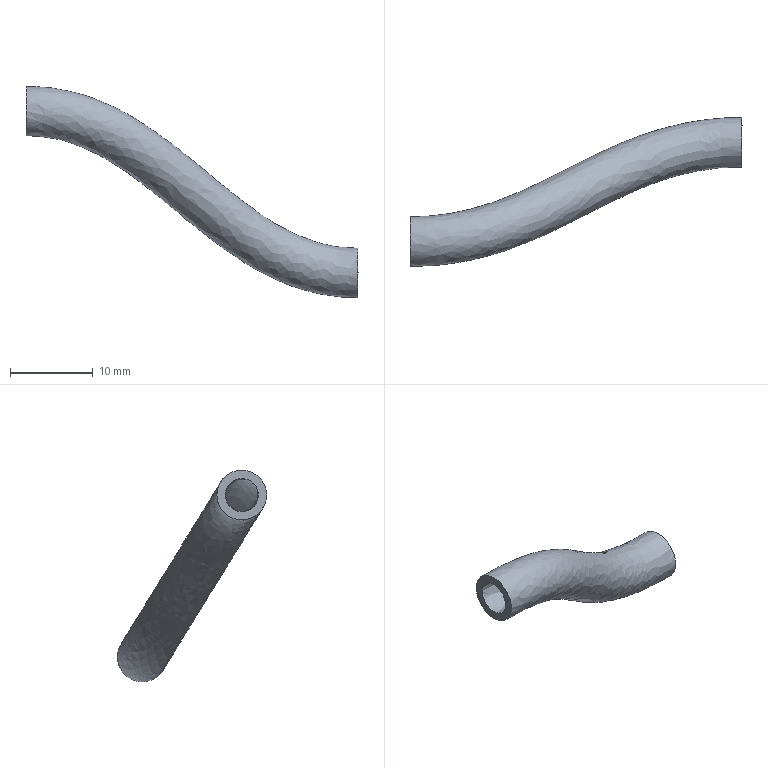Part | NX | features solid 2 | 1 solid | 4 faces | box 40 x 18 x 25.5 mm | volume 744.374 mm3 | plane 2 | spline 2